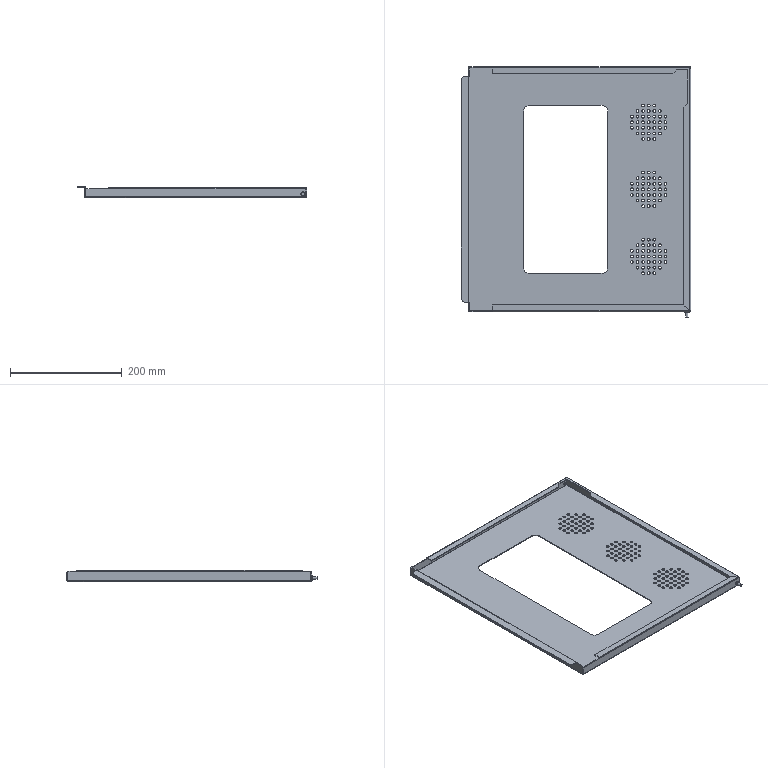Part | STEP file | FHD-021-014-A front door B | 1 solid | 214 faces | box 410 x 447 x 20 mm | volume 253871 mm3 | cylinder 137 | plane 69 | spline 8 | commonest cylinder face diameters 5 x114 0.4 x8 3.4 x8 20 x4 15 x2 7.8 x1